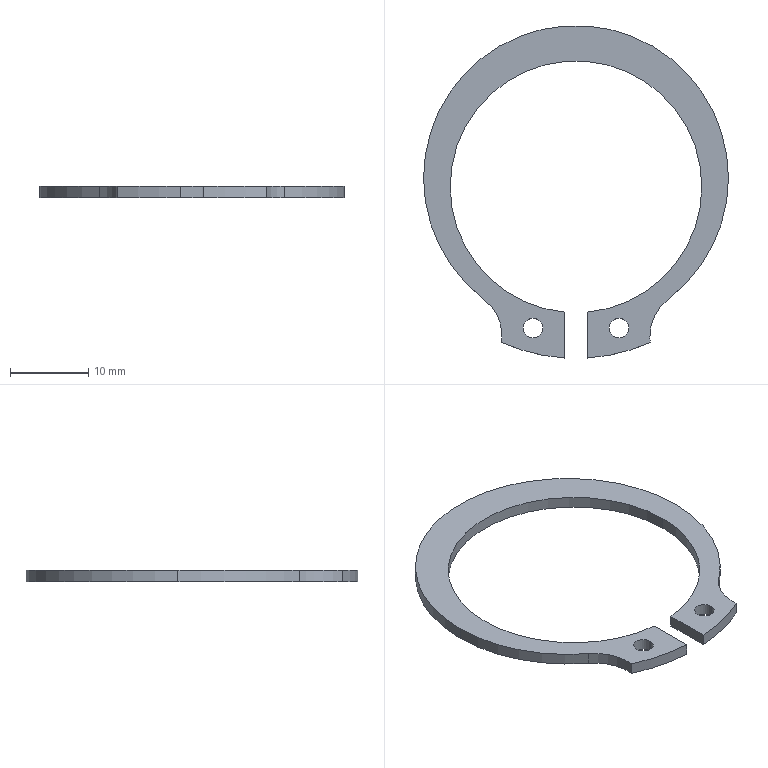Part | STEP file | GB894.2-86 shaft elastic retaining ring type B 35 | 1 solid | 19 faces | box 39 x 42.531 x 1.5 mm | volume 639.019 mm3 | cylinder 15 | plane 4 | commonest cylinder face diameters 2.5 x4 12 x3 32.2 x3 39 x3 46.16 x2